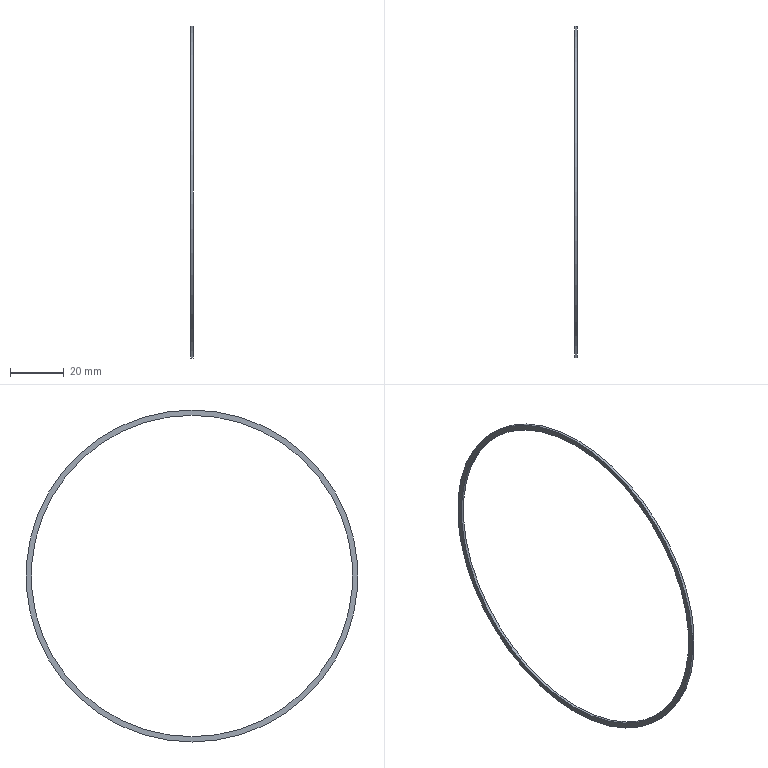Part | STEP file | Sealing ring | 1 solid | 4 faces | box 1 x 124 x 124 mm | volume 766.549 mm3 | plane 2 | cylinder 2 | commonest cylinder face diameters 120 x1 124 x1
STEP:
#1=CARTESIAN_POINT('',(0.,0.,-62.));
#2=VERTEX_POINT('',#1);
#3=CARTESIAN_POINT('',(0.,0.,0.));
#4=DIRECTION('',(1.,0.,0.));
#5=DIRECTION('',(0.,0.,-1.));
#6=AXIS2_PLACEMENT_3D('',#3,#4,#5);
#7=CIRCLE('',#6,62.);
#8=EDGE_CURVE('',#2,#2,#7,.T.);
#9=ORIENTED_EDGE('',*,*,#8,.F.);
#10=EDGE_LOOP('',(#9));
#11=FACE_BOUND('',#10,.T.);
#12=CARTESIAN_POINT('',(0.,0.,-60.));
#13=VERTEX_POINT('',#12);
#14=CARTESIAN_POINT('',(0.,0.,0.));
#15=DIRECTION('',(1.,0.,0.));
#16=DIRECTION('',(0.,0.,-1.));
#17=AXIS2_PLACEMENT_3D('',#14,#15,#16);
#18=CIRCLE('',#17,60.);
#19=EDGE_CURVE('',#13,#13,#18,.T.);
#20=ORIENTED_EDGE('',*,*,#19,.T.);
#21=EDGE_LOOP('',(#20));
#22=FACE_BOUND('',#21,.T.);
#23=CARTESIAN_POINT('',(0.,0.,0.));
#24=DIRECTION('',(1.,0.,0.));
#25=DIRECTION('',(0.,0.,-1.));
#26=AXIS2_PLACEMENT_3D('',#23,#24,#25);
#27=PLANE('',#26);
#28=ADVANCED_FACE('',(#11,#22),#27,.F.);
#29=CARTESIAN_POINT('',(1.,0.,-62.));
#30=VERTEX_POINT('',#29);
#31=CARTESIAN_POINT('',(1.,0.,0.));
#32=DIRECTION('',(1.,0.,0.));
#33=DIRECTION('',(0.,0.,-1.));
#34=AXIS2_PLACEMENT_3D('',#31,#32,#33);
#35=CIRCLE('',#34,62.);
#36=EDGE_CURVE('',#30,#30,#35,.T.);
#37=ORIENTED_EDGE('',*,*,#36,.T.);
#38=EDGE_LOOP('',(#37));
#39=FACE_BOUND('',#38,.T.);
#40=CARTESIAN_POINT('',(1.,0.,-60.));
#41=VERTEX_POINT('',#40);
#42=CARTESIAN_POINT('',(1.,0.,0.));
#43=DIRECTION('',(1.,0.,0.));
#44=DIRECTION('',(0.,0.,-1.));
#45=AXIS2_PLACEMENT_3D('',#42,#43,#44);
#46=CIRCLE('',#45,60.);
#47=EDGE_CURVE('',#41,#41,#46,.F.);
#48=ORIENTED_EDGE('',*,*,#47,.T.);
#49=EDGE_LOOP('',(#48));
#50=FACE_BOUND('',#49,.T.);
#51=CARTESIAN_POINT('',(1.,0.,0.));
#52=DIRECTION('',(1.,0.,0.));
#53=DIRECTION('',(0.,0.,-1.));
#54=AXIS2_PLACEMENT_3D('',#51,#52,#53);
#55=PLANE('',#54);
#56=ADVANCED_FACE('',(#39,#50),#55,.T.);
#57=ORIENTED_EDGE('',*,*,#47,.F.);
#58=EDGE_LOOP('',(#57));
#59=FACE_OUTER_BOUND('',#58,.T.);
#60=ORIENTED_EDGE('',*,*,#19,.F.);
#61=EDGE_LOOP('',(#60));
#62=FACE_OUTER_BOUND('',#61,.T.);
#63=CARTESIAN_POINT('',(0.,0.,0.));
#64=DIRECTION('',(1.,0.,0.));
#65=DIRECTION('',(0.,0.,-1.));
#66=AXIS2_PLACEMENT_3D('',#63,#64,#65);
#67=CYLINDRICAL_SURFACE('',#66,60.);
#68=ADVANCED_FACE('',(#59,#62),#67,.F.);
#69=ORIENTED_EDGE('',*,*,#36,.F.);
#70=EDGE_LOOP('',(#69));
#71=FACE_OUTER_BOUND('',#70,.T.);
#72=ORIENTED_EDGE('',*,*,#8,.T.);
#73=EDGE_LOOP('',(#72));
#74=FACE_OUTER_BOUND('',#73,.T.);
#75=CARTESIAN_POINT('',(0.,0.,0.));
#76=DIRECTION('',(1.,0.,0.));
#77=DIRECTION('',(0.,0.,-1.));
#78=AXIS2_PLACEMENT_3D('',#75,#76,#77);
#79=CYLINDRICAL_SURFACE('',#78,62.);
#80=ADVANCED_FACE('',(#71,#74),#79,.T.);
#81=CLOSED_SHELL('',(#28,#56,#68,#80));
#82=MANIFOLD_SOLID_BREP('',#81);
#83=(LENGTH_UNIT()NAMED_UNIT(*)SI_UNIT(.MILLI.,.METRE.));
#84=UNCERTAINTY_MEASURE_WITH_UNIT(LENGTH_MEASURE(0.00001),#83,'','');
#85=(NAMED_UNIT(*)PLANE_ANGLE_UNIT()SI_UNIT($,.RADIAN.));
#86=(NAMED_UNIT(*)SI_UNIT($,.STERADIAN.)SOLID_ANGLE_UNIT());
#87=(GEOMETRIC_REPRESENTATION_CONTEXT(3)GLOBAL_UNCERTAINTY_ASSIGNED_CONTEXT((#84))GLOBAL_UNIT_ASSIGNED_CONTEXT((#83,#85,#86))REPRESENTATION_CONTEXT('',''));
#88=ADVANCED_BREP_SHAPE_REPRESENTATION('',(#82),#87);